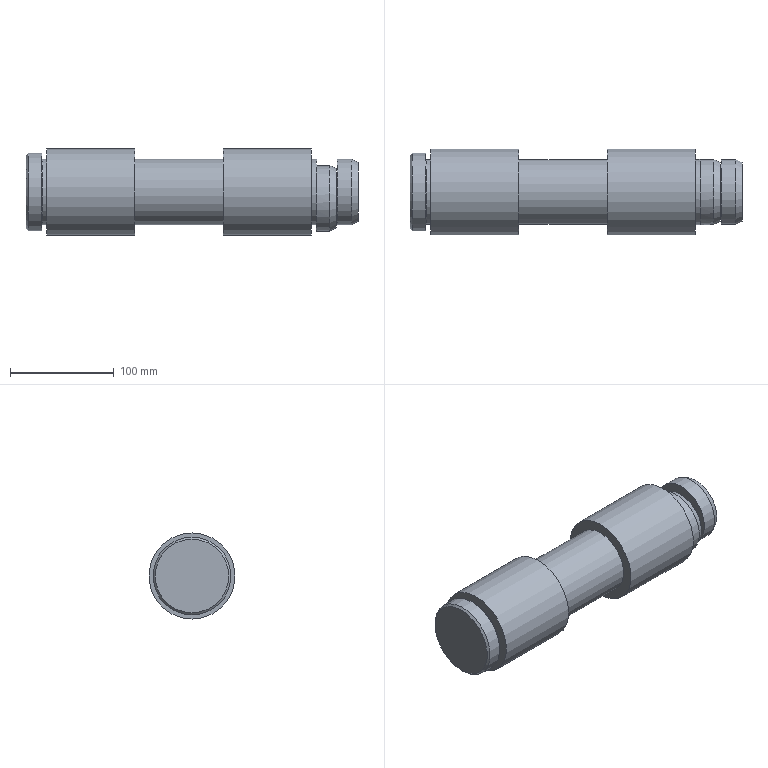Part | NX | features solid 2 | 1 solid | 36 faces | box 320 x 83 x 83 mm | volume 1384742 mm3 | plane 14 | cylinder 12 | cone 7 | torus 3 | commonest cylinder face diameters 63 x5 83 x2 27 x1 27.2 x1 32 x1 44 x1
STEP:
#1=CARTESIAN_POINT('',(-1305.,-953.648,-403.05));
#2=VERTEX_POINT('',#1);
#3=CARTESIAN_POINT('',(-1305.,-1016.352,-403.05));
#4=VERTEX_POINT('',#3);
#5=CARTESIAN_POINT('',(-1305.,-985.,-406.1));
#6=DIRECTION('',(1.,0.,0.));
#7=DIRECTION('',(0.,0.,-1.));
#8=AXIS2_PLACEMENT_3D('',#5,#6,#7);
#9=CIRCLE('',#8,31.5);
#10=EDGE_CURVE('',#2,#4,#9,.T.);
#11=ORIENTED_EDGE('',*,*,#10,.F.);
#12=CARTESIAN_POINT('',(-1305.,-985.,-400.));
#13=DIRECTION('',(1.,0.,0.));
#14=DIRECTION('',(0.,0.,1.));
#15=AXIS2_PLACEMENT_3D('',#12,#13,#14);
#16=CIRCLE('',#15,31.5);
#17=EDGE_CURVE('',#2,#4,#16,.T.);
#18=ORIENTED_EDGE('',*,*,#17,.T.);
#19=EDGE_LOOP('',(#11,#18));
#20=FACE_BOUND('',#19,.T.);
#21=CARTESIAN_POINT('',(-1305.,-985.,-400.));
#22=DIRECTION('',(1.,0.,0.));
#23=DIRECTION('',(0.,0.,1.));
#24=AXIS2_PLACEMENT_3D('',#21,#22,#23);
#25=PLANE('',#24);
#26=ADVANCED_FACE('',(#20),#25,.T.);
#27=CARTESIAN_POINT('',(-1310.,-985.,-431.5));
#28=VERTEX_POINT('',#27);
#29=CARTESIAN_POINT('',(-1310.,-985.,-400.));
#30=DIRECTION('',(1.,0.,0.));
#31=DIRECTION('',(0.,0.,-1.));
#32=AXIS2_PLACEMENT_3D('',#29,#30,#31);
#33=CIRCLE('',#32,31.5);
#34=EDGE_CURVE('',#28,#28,#33,.F.);
#35=ORIENTED_EDGE('',*,*,#34,.F.);
#36=EDGE_LOOP('',(#35));
#37=FACE_BOUND('',#36,.T.);
#38=CARTESIAN_POINT('',(-1305.,-985.,-400.));
#39=DIRECTION('',(1.,0.,0.));
#40=DIRECTION('',(0.,0.,1.));
#41=AXIS2_PLACEMENT_3D('',#38,#39,#40);
#42=CIRCLE('',#41,31.5);
#43=EDGE_CURVE('',#4,#2,#42,.T.);
#44=ORIENTED_EDGE('',*,*,#43,.F.);
#45=ORIENTED_EDGE('',*,*,#17,.F.);
#46=EDGE_LOOP('',(#44,#45));
#47=FACE_BOUND('',#46,.T.);
#48=CARTESIAN_POINT('',(-1570.,-985.,-400.));
#49=DIRECTION('',(1.,0.,0.));
#50=DIRECTION('',(0.,0.,1.));
#51=AXIS2_PLACEMENT_3D('',#48,#49,#50);
#52=CYLINDRICAL_SURFACE('',#51,31.5);
#53=ADVANCED_FACE('',(#37,#47),#52,.T.);
#54=ORIENTED_EDGE('',*,*,#34,.T.);
#55=EDGE_LOOP('',(#54));
#56=FACE_BOUND('',#55,.T.);
#57=CARTESIAN_POINT('',(-1310.,-985.,-441.5));
#58=VERTEX_POINT('',#57);
#59=CARTESIAN_POINT('',(-1310.,-985.,-400.));
#60=DIRECTION('',(-1.,0.,0.));
#61=DIRECTION('',(0.,0.,-1.));
#62=AXIS2_PLACEMENT_3D('',#59,#60,#61);
#63=CIRCLE('',#62,41.5);
#64=EDGE_CURVE('',#58,#58,#63,.T.);
#65=ORIENTED_EDGE('',*,*,#64,.F.);
#66=EDGE_LOOP('',(#65));
#67=FACE_BOUND('',#66,.T.);
#68=CARTESIAN_POINT('',(-1310.,-985.,-400.));
#69=DIRECTION('',(1.,0.,0.));
#70=DIRECTION('',(0.,0.,1.));
#71=AXIS2_PLACEMENT_3D('',#68,#69,#70);
#72=PLANE('',#71);
#73=ADVANCED_FACE('',(#56,#67),#72,.T.);
#74=CARTESIAN_POINT('',(-1395.,-985.,-368.5));
#75=VERTEX_POINT('',#74);
#76=CARTESIAN_POINT('',(-1395.,-985.,-400.));
#77=DIRECTION('',(-1.,0.,0.));
#78=DIRECTION('',(0.,0.,1.));
#79=AXIS2_PLACEMENT_3D('',#76,#77,#78);
#80=CIRCLE('',#79,31.5);
#81=EDGE_CURVE('',#75,#75,#80,.F.);
#82=ORIENTED_EDGE('',*,*,#81,.T.);
#83=EDGE_LOOP('',(#82));
#84=FACE_BOUND('',#83,.T.);
#85=CARTESIAN_POINT('',(-1395.,-985.,-358.5));
#86=VERTEX_POINT('',#85);
#87=CARTESIAN_POINT('',(-1395.,-985.,-400.));
#88=DIRECTION('',(1.,0.,0.));
#89=DIRECTION('',(0.,0.,1.));
#90=AXIS2_PLACEMENT_3D('',#87,#88,#89);
#91=CIRCLE('',#90,41.5);
#92=EDGE_CURVE('',#86,#86,#91,.T.);
#93=ORIENTED_EDGE('',*,*,#92,.F.);
#94=EDGE_LOOP('',(#93));
#95=FACE_BOUND('',#94,.T.);
#96=CARTESIAN_POINT('',(-1395.,-985.,-400.));
#97=DIRECTION('',(-1.,0.,0.));
#98=DIRECTION('',(0.,0.,-1.));
#99=AXIS2_PLACEMENT_3D('',#96,#97,#98);
#100=PLANE('',#99);
#101=ADVANCED_FACE('',(#84,#95),#100,.T.);
#102=ORIENTED_EDGE('',*,*,#64,.T.);
#103=EDGE_LOOP('',(#102));
#104=FACE_BOUND('',#103,.T.);
#105=ORIENTED_EDGE('',*,*,#92,.T.);
#106=EDGE_LOOP('',(#105));
#107=FACE_BOUND('',#106,.T.);
#108=CARTESIAN_POINT('',(-1395.,-985.,-400.));
#109=DIRECTION('',(1.,0.,0.));
#110=DIRECTION('',(0.,0.,1.));
#111=AXIS2_PLACEMENT_3D('',#108,#109,#110);
#112=CYLINDRICAL_SURFACE('',#111,41.5);
#113=ADVANCED_FACE('',(#104,#107),#112,.T.);
#114=CARTESIAN_POINT('',(-1585.,-985.,-364.5));
#115=VERTEX_POINT('',#114);
#116=CARTESIAN_POINT('',(-1585.,-985.,-400.));
#117=DIRECTION('',(-1.,0.,0.));
#118=DIRECTION('',(0.,0.,1.));
#119=AXIS2_PLACEMENT_3D('',#116,#117,#118);
#120=CIRCLE('',#119,35.5);
#121=EDGE_CURVE('',#115,#115,#120,.T.);
#122=ORIENTED_EDGE('',*,*,#121,.T.);
#123=EDGE_LOOP('',(#122));
#124=FACE_BOUND('',#123,.T.);
#125=CARTESIAN_POINT('',(-1585.,-985.,-400.));
#126=DIRECTION('',(-1.,0.,0.));
#127=DIRECTION('',(0.,0.,-1.));
#128=AXIS2_PLACEMENT_3D('',#125,#126,#127);
#129=PLANE('',#128);
#130=ADVANCED_FACE('',(#124),#129,.T.);
#131=ORIENTED_EDGE('',*,*,#121,.F.);
#132=EDGE_LOOP('',(#131));
#133=FACE_BOUND('',#132,.T.);
#134=CARTESIAN_POINT('',(-1583.,-985.,-362.5));
#135=VERTEX_POINT('',#134);
#136=CARTESIAN_POINT('',(-1583.,-985.,-400.));
#137=DIRECTION('',(-1.,0.,0.));
#138=DIRECTION('',(0.,0.,1.));
#139=AXIS2_PLACEMENT_3D('',#136,#137,#138);
#140=CIRCLE('',#139,37.5);
#141=EDGE_CURVE('',#135,#135,#140,.F.);
#142=ORIENTED_EDGE('',*,*,#141,.F.);
#143=EDGE_LOOP('',(#142));
#144=FACE_BOUND('',#143,.T.);
#145=CARTESIAN_POINT('',(-1583.,-985.,-400.));
#146=DIRECTION('',(1.,0.,0.));
#147=DIRECTION('',(0.,0.,-1.));
#148=AXIS2_PLACEMENT_3D('',#145,#146,#147);
#149=CONICAL_SURFACE('',#148,37.5,0.7854);
#150=ADVANCED_FACE('',(#133,#144),#149,.T.);
#151=ORIENTED_EDGE('',*,*,#141,.T.);
#152=EDGE_LOOP('',(#151));
#153=FACE_BOUND('',#152,.T.);
#154=CARTESIAN_POINT('',(-1570.,-985.,-437.5));
#155=VERTEX_POINT('',#154);
#156=CARTESIAN_POINT('',(-1570.,-985.,-400.));
#157=DIRECTION('',(-1.,0.,0.));
#158=DIRECTION('',(0.,0.,-1.));
#159=AXIS2_PLACEMENT_3D('',#156,#157,#158);
#160=CIRCLE('',#159,37.5);
#161=EDGE_CURVE('',#155,#155,#160,.T.);
#162=ORIENTED_EDGE('',*,*,#161,.T.);
#163=EDGE_LOOP('',(#162));
#164=FACE_BOUND('',#163,.T.);
#165=CARTESIAN_POINT('',(-1585.,-985.,-400.));
#166=DIRECTION('',(1.,0.,0.));
#167=DIRECTION('',(0.,0.,1.));
#168=AXIS2_PLACEMENT_3D('',#165,#166,#167);
#169=CYLINDRICAL_SURFACE('',#168,37.5);
#170=ADVANCED_FACE('',(#153,#164),#169,.T.);
#171=CARTESIAN_POINT('',(-1570.,-985.,-432.5));
#172=VERTEX_POINT('',#171);
#173=CARTESIAN_POINT('',(-1570.,-985.,-400.));
#174=DIRECTION('',(1.,0.,0.));
#175=DIRECTION('',(0.,0.,-1.));
#176=AXIS2_PLACEMENT_3D('',#173,#174,#175);
#177=CIRCLE('',#176,32.5);
#178=EDGE_CURVE('',#172,#172,#177,.F.);
#179=ORIENTED_EDGE('',*,*,#178,.T.);
#180=EDGE_LOOP('',(#179));
#181=FACE_BOUND('',#180,.T.);
#182=ORIENTED_EDGE('',*,*,#161,.F.);
#183=EDGE_LOOP('',(#182));
#184=FACE_BOUND('',#183,.T.);
#185=CARTESIAN_POINT('',(-1570.,-985.,-400.));
#186=DIRECTION('',(1.,0.,0.));
#187=DIRECTION('',(0.,0.,1.));
#188=AXIS2_PLACEMENT_3D('',#185,#186,#187);
#189=PLANE('',#188);
#190=ADVANCED_FACE('',(#181,#184),#189,.T.);
#191=ORIENTED_EDGE('',*,*,#178,.F.);
#192=EDGE_LOOP('',(#191));
#193=FACE_BOUND('',#192,.T.);
#194=CARTESIAN_POINT('',(-1569.,-985.,-431.5));
#195=VERTEX_POINT('',#194);
#196=CARTESIAN_POINT('',(-1569.,-985.,-400.));
#197=DIRECTION('',(1.,0.,0.));
#198=DIRECTION('',(0.,0.,-1.));
#199=AXIS2_PLACEMENT_3D('',#196,#197,#198);
#200=CIRCLE('',#199,31.5);
#201=EDGE_CURVE('',#195,#195,#200,.T.);
#202=ORIENTED_EDGE('',*,*,#201,.F.);
#203=EDGE_LOOP('',(#202));
#204=FACE_BOUND('',#203,.T.);
#205=CARTESIAN_POINT('',(-1569.,-985.,-400.));
#206=DIRECTION('',(1.,0.,0.));
#207=DIRECTION('',(0.,0.,-1.));
#208=AXIS2_PLACEMENT_3D('',#205,#206,#207);
#209=TOROIDAL_SURFACE('',#208,32.5,1.);
#210=ADVANCED_FACE('',(#193,#204),#209,.F.);
#211=CARTESIAN_POINT('',(-1565.,-985.,-368.5));
#212=VERTEX_POINT('',#211);
#213=CARTESIAN_POINT('',(-1565.,-985.,-400.));
#214=DIRECTION('',(-1.,0.,0.));
#215=DIRECTION('',(0.,0.,1.));
#216=AXIS2_PLACEMENT_3D('',#213,#214,#215);
#217=CIRCLE('',#216,31.5);
#218=EDGE_CURVE('',#212,#212,#217,.F.);
#219=ORIENTED_EDGE('',*,*,#218,.F.);
#220=EDGE_LOOP('',(#219));
#221=FACE_BOUND('',#220,.T.);
#222=ORIENTED_EDGE('',*,*,#201,.T.);
#223=EDGE_LOOP('',(#222));
#224=FACE_BOUND('',#223,.T.);
#225=CARTESIAN_POINT('',(-1570.,-985.,-400.));
#226=DIRECTION('',(1.,0.,0.));
#227=DIRECTION('',(0.,0.,1.));
#228=AXIS2_PLACEMENT_3D('',#225,#226,#227);
#229=CYLINDRICAL_SURFACE('',#228,31.5);
#230=ADVANCED_FACE('',(#221,#224),#229,.T.);
#231=ORIENTED_EDGE('',*,*,#218,.T.);
#232=EDGE_LOOP('',(#231));
#233=FACE_BOUND('',#232,.T.);
#234=CARTESIAN_POINT('',(-1565.,-985.,-358.5));
#235=VERTEX_POINT('',#234);
#236=CARTESIAN_POINT('',(-1565.,-985.,-400.));
#237=DIRECTION('',(1.,0.,0.));
#238=DIRECTION('',(0.,0.,1.));
#239=AXIS2_PLACEMENT_3D('',#236,#237,#238);
#240=CIRCLE('',#239,41.5);
#241=EDGE_CURVE('',#235,#235,#240,.T.);
#242=ORIENTED_EDGE('',*,*,#241,.F.);
#243=EDGE_LOOP('',(#242));
#244=FACE_BOUND('',#243,.T.);
#245=CARTESIAN_POINT('',(-1565.,-985.,-400.));
#246=DIRECTION('',(-1.,0.,0.));
#247=DIRECTION('',(0.,0.,-1.));
#248=AXIS2_PLACEMENT_3D('',#245,#246,#247);
#249=PLANE('',#248);
#250=ADVANCED_FACE('',(#233,#244),#249,.T.);
#251=CARTESIAN_POINT('',(-1480.,-985.,-441.5));
#252=VERTEX_POINT('',#251);
#253=CARTESIAN_POINT('',(-1480.,-985.,-400.));
#254=DIRECTION('',(-1.,0.,0.));
#255=DIRECTION('',(0.,0.,-1.));
#256=AXIS2_PLACEMENT_3D('',#253,#254,#255);
#257=CIRCLE('',#256,41.5);
#258=EDGE_CURVE('',#252,#252,#257,.T.);
#259=ORIENTED_EDGE('',*,*,#258,.T.);
#260=EDGE_LOOP('',(#259));
#261=FACE_BOUND('',#260,.T.);
#262=ORIENTED_EDGE('',*,*,#241,.T.);
#263=EDGE_LOOP('',(#262));
#264=FACE_BOUND('',#263,.T.);
#265=CARTESIAN_POINT('',(-1565.,-985.,-400.));
#266=DIRECTION('',(1.,0.,0.));
#267=DIRECTION('',(0.,0.,1.));
#268=AXIS2_PLACEMENT_3D('',#265,#266,#267);
#269=CYLINDRICAL_SURFACE('',#268,41.5);
#270=ADVANCED_FACE('',(#261,#264),#269,.T.);
#271=CARTESIAN_POINT('',(-1480.,-985.,-431.5));
#272=VERTEX_POINT('',#271);
#273=CARTESIAN_POINT('',(-1480.,-985.,-400.));
#274=DIRECTION('',(1.,0.,0.));
#275=DIRECTION('',(0.,0.,-1.));
#276=AXIS2_PLACEMENT_3D('',#273,#274,#275);
#277=CIRCLE('',#276,31.5);
#278=EDGE_CURVE('',#272,#272,#277,.F.);
#279=ORIENTED_EDGE('',*,*,#278,.T.);
#280=EDGE_LOOP('',(#279));
#281=FACE_BOUND('',#280,.T.);
#282=ORIENTED_EDGE('',*,*,#258,.F.);
#283=EDGE_LOOP('',(#282));
#284=FACE_BOUND('',#283,.T.);
#285=CARTESIAN_POINT('',(-1480.,-985.,-400.));
#286=DIRECTION('',(1.,0.,0.));
#287=DIRECTION('',(0.,0.,1.));
#288=AXIS2_PLACEMENT_3D('',#285,#286,#287);
#289=PLANE('',#288);
#290=ADVANCED_FACE('',(#281,#284),#289,.T.);
#291=ORIENTED_EDGE('',*,*,#81,.F.);
#292=EDGE_LOOP('',(#291));
#293=FACE_BOUND('',#292,.T.);
#294=ORIENTED_EDGE('',*,*,#278,.F.);
#295=EDGE_LOOP('',(#294));
#296=FACE_BOUND('',#295,.T.);
#297=CARTESIAN_POINT('',(-1570.,-985.,-400.));
#298=DIRECTION('',(1.,0.,0.));
#299=DIRECTION('',(0.,0.,1.));
#300=AXIS2_PLACEMENT_3D('',#297,#298,#299);
#301=CYLINDRICAL_SURFACE('',#300,31.5);
#302=ADVANCED_FACE('',(#293,#296),#301,.T.);
#303=CARTESIAN_POINT('',(-1286.,-985.,-434.6));
#304=VERTEX_POINT('',#303);
#305=CARTESIAN_POINT('',(-1286.,-985.,-406.1));
#306=DIRECTION('',(1.,0.,0.));
#307=DIRECTION('',(0.,0.,-1.));
#308=AXIS2_PLACEMENT_3D('',#305,#306,#307);
#309=CIRCLE('',#308,28.5);
#310=EDGE_CURVE('',#304,#304,#309,.T.);
#311=ORIENTED_EDGE('',*,*,#310,.T.);
#312=EDGE_LOOP('',(#311));
#313=FACE_BOUND('',#312,.T.);
#314=CARTESIAN_POINT('',(-1286.,-981.618,-384.361));
#315=VERTEX_POINT('',#314);
#316=CARTESIAN_POINT('',(-1286.,-988.382,-384.361));
#317=VERTEX_POINT('',#316);
#318=CARTESIAN_POINT('',(-1286.,-985.,-406.1));
#319=DIRECTION('',(-1.,0.,0.));
#320=DIRECTION('',(0.,0.,-1.));
#321=AXIS2_PLACEMENT_3D('',#318,#319,#320);
#322=CIRCLE('',#321,22.);
#323=EDGE_CURVE('',#315,#317,#322,.T.);
#324=ORIENTED_EDGE('',*,*,#323,.T.);
#325=CARTESIAN_POINT('',(-1286.,-985.,-400.));
#326=DIRECTION('',(1.,0.,0.));
#327=DIRECTION('',(0.,0.,-1.));
#328=AXIS2_PLACEMENT_3D('',#325,#326,#327);
#329=CIRCLE('',#328,16.);
#330=EDGE_CURVE('',#317,#315,#329,.F.);
#331=ORIENTED_EDGE('',*,*,#330,.T.);
#332=EDGE_LOOP('',(#324,#331));
#333=FACE_BOUND('',#332,.T.);
#334=CARTESIAN_POINT('',(-1286.,-985.,-406.1));
#335=DIRECTION('',(1.,0.,0.));
#336=DIRECTION('',(0.,0.,1.));
#337=AXIS2_PLACEMENT_3D('',#334,#335,#336);
#338=PLANE('',#337);
#339=ADVANCED_FACE('',(#313,#333),#338,.T.);
#340=CARTESIAN_POINT('',(-1305.,-985.,-406.1));
#341=DIRECTION('',(1.,0.,0.));
#342=DIRECTION('',(0.,0.,1.));
#343=AXIS2_PLACEMENT_3D('',#340,#341,#342);
#344=CIRCLE('',#343,31.5);
#345=EDGE_CURVE('',#4,#2,#344,.T.);
#346=ORIENTED_EDGE('',*,*,#345,.F.);
#347=ORIENTED_EDGE('',*,*,#43,.T.);
#348=EDGE_LOOP('',(#346,#347));
#349=FACE_BOUND('',#348,.T.);
#350=CARTESIAN_POINT('',(-1305.,-985.,-406.1));
#351=DIRECTION('',(-1.,0.,0.));
#352=DIRECTION('',(0.,0.,-1.));
#353=AXIS2_PLACEMENT_3D('',#350,#351,#352);
#354=PLANE('',#353);
#355=ADVANCED_FACE('',(#349),#354,.T.);
#356=CARTESIAN_POINT('',(-1292.,-985.,-437.6));
#357=VERTEX_POINT('',#356);
#358=CARTESIAN_POINT('',(-1292.,-985.,-406.1));
#359=DIRECTION('',(1.,0.,0.));
#360=DIRECTION('',(0.,0.,-1.));
#361=AXIS2_PLACEMENT_3D('',#358,#359,#360);
#362=CIRCLE('',#361,31.5);
#363=EDGE_CURVE('',#357,#357,#362,.F.);
#364=ORIENTED_EDGE('',*,*,#363,.T.);
#365=EDGE_LOOP('',(#364));
#366=FACE_BOUND('',#365,.T.);
#367=ORIENTED_EDGE('',*,*,#345,.T.);
#368=ORIENTED_EDGE('',*,*,#10,.T.);
#369=EDGE_LOOP('',(#367,#368));
#370=FACE_BOUND('',#369,.T.);
#371=CARTESIAN_POINT('',(-1305.,-985.,-406.1));
#372=DIRECTION('',(1.,0.,0.));
#373=DIRECTION('',(0.,0.,1.));
#374=AXIS2_PLACEMENT_3D('',#371,#372,#373);
#375=CYLINDRICAL_SURFACE('',#374,31.5);
#376=ADVANCED_FACE('',(#366,#370),#375,.T.);
#377=CARTESIAN_POINT('',(-1304.2,-981.618,-384.361));
#378=VERTEX_POINT('',#377);
#379=CARTESIAN_POINT('',(-1295.1,-981.618,-384.361));
#380=DIRECTION('',(-1.,0.,0.));
#381=VECTOR('',#380,1000.);
#382=LINE('',#379,#381);
#383=EDGE_CURVE('',#378,#315,#382,.F.);
#384=ORIENTED_EDGE('',*,*,#383,.F.);
#385=CARTESIAN_POINT('',(-1304.2,-988.382,-384.361));
#386=VERTEX_POINT('',#385);
#387=CARTESIAN_POINT('',(-1304.2,-985.,-406.1));
#388=DIRECTION('',(-1.,0.,0.));
#389=DIRECTION('',(0.,0.,1.));
#390=AXIS2_PLACEMENT_3D('',#387,#388,#389);
#391=CIRCLE('',#390,22.);
#392=EDGE_CURVE('',#378,#386,#391,.T.);
#393=ORIENTED_EDGE('',*,*,#392,.T.);
#394=CARTESIAN_POINT('',(-1295.1,-988.382,-384.361));
#395=DIRECTION('',(-1.,0.,0.));
#396=VECTOR('',#395,1000.);
#397=LINE('',#394,#396);
#398=EDGE_CURVE('',#317,#386,#397,.T.);
#399=ORIENTED_EDGE('',*,*,#398,.F.);
#400=ORIENTED_EDGE('',*,*,#323,.F.);
#401=EDGE_LOOP('',(#384,#393,#399,#400));
#402=FACE_BOUND('',#401,.T.);
#403=CARTESIAN_POINT('',(-1286.,-985.,-406.1));
#404=DIRECTION('',(-1.,0.,0.));
#405=DIRECTION('',(0.,0.,-1.));
#406=AXIS2_PLACEMENT_3D('',#403,#404,#405);
#407=CYLINDRICAL_SURFACE('',#406,22.);
#408=ADVANCED_FACE('',(#402),#407,.F.);
#409=CARTESIAN_POINT('',(-1305.,-985.,-428.9));
#410=VERTEX_POINT('',#409);
#411=CARTESIAN_POINT('',(-1305.,-985.,-406.1));
#412=DIRECTION('',(1.,0.,0.));
#413=DIRECTION('',(0.,0.,-1.));
#414=AXIS2_PLACEMENT_3D('',#411,#412,#413);
#415=CIRCLE('',#414,22.8);
#416=EDGE_CURVE('',#410,#410,#415,.F.);
#417=ORIENTED_EDGE('',*,*,#416,.T.);
#418=EDGE_LOOP('',(#417));
#419=FACE_BOUND('',#418,.T.);
#420=ORIENTED_EDGE('',*,*,#392,.F.);
#421=CARTESIAN_POINT('',(-1304.2,-981.618,-384.361));
#422=CARTESIAN_POINT('',(-1304.334,-983.853,-383.878));
#423=CARTESIAN_POINT('',(-1304.334,-986.147,-383.878));
#424=CARTESIAN_POINT('',(-1304.2,-988.382,-384.361));
#425=B_SPLINE_CURVE_WITH_KNOTS('',3,(#421,#422,#423,#424),.UNSPECIFIED.,.F.,.F.,(4,4),(0.000003368,0.006776),.UNSPECIFIED.);
#426=EDGE_CURVE('',#378,#386,#425,.T.);
#427=ORIENTED_EDGE('',*,*,#426,.T.);
#428=EDGE_LOOP('',(#420,#427));
#429=FACE_BOUND('',#428,.T.);
#430=CARTESIAN_POINT('',(-1304.2,-985.,-406.1));
#431=DIRECTION('',(-1.,0.,0.));
#432=DIRECTION('',(0.,0.,1.));
#433=AXIS2_PLACEMENT_3D('',#430,#431,#432);
#434=CONICAL_SURFACE('',#433,22.,0.7854);
#435=ADVANCED_FACE('',(#419,#429),#434,.F.);
#436=ORIENTED_EDGE('',*,*,#310,.F.);
#437=EDGE_LOOP('',(#436));
#438=FACE_BOUND('',#437,.T.);
#439=ORIENTED_EDGE('',*,*,#363,.F.);
#440=EDGE_LOOP('',(#439));
#441=FACE_BOUND('',#440,.T.);
#442=CARTESIAN_POINT('',(-1292.,-985.,-406.1));
#443=DIRECTION('',(-1.,0.,0.));
#444=DIRECTION('',(0.,0.,1.));
#445=AXIS2_PLACEMENT_3D('',#442,#443,#444);
#446=CONICAL_SURFACE('',#445,31.5,0.4636);
#447=ADVANCED_FACE('',(#438,#441),#446,.T.);
#448=CARTESIAN_POINT('',(-1265.,-985.,-408.5));
#449=VERTEX_POINT('',#448);
#450=CARTESIAN_POINT('',(-1265.,-985.,-400.));
#451=DIRECTION('',(1.,0.,0.));
#452=DIRECTION('',(0.,0.,-1.));
#453=AXIS2_PLACEMENT_3D('',#450,#451,#452);
#454=CIRCLE('',#453,8.5);
#455=EDGE_CURVE('',#449,#449,#454,.T.);
#456=ORIENTED_EDGE('',*,*,#455,.T.);
#457=EDGE_LOOP('',(#456));
#458=FACE_BOUND('',#457,.T.);
#459=CARTESIAN_POINT('',(-1265.,-985.,-400.));
#460=DIRECTION('',(1.,0.,0.));
#461=DIRECTION('',(0.,0.,1.));
#462=AXIS2_PLACEMENT_3D('',#459,#460,#461);
#463=PLANE('',#462);
#464=ADVANCED_FACE('',(#458),#463,.T.);
#465=CARTESIAN_POINT('',(-1270.,-985.,-413.5));
#466=VERTEX_POINT('',#465);
#467=CARTESIAN_POINT('',(-1270.,-985.,-400.));
#468=DIRECTION('',(1.,0.,0.));
#469=DIRECTION('',(0.,0.,-1.));
#470=AXIS2_PLACEMENT_3D('',#467,#468,#469);
#471=CIRCLE('',#470,13.5);
#472=EDGE_CURVE('',#466,#466,#471,.F.);
#473=ORIENTED_EDGE('',*,*,#472,.F.);
#474=EDGE_LOOP('',(#473));
#475=FACE_BOUND('',#474,.T.);
#476=ORIENTED_EDGE('',*,*,#455,.F.);
#477=EDGE_LOOP('',(#476));
#478=FACE_BOUND('',#477,.T.);
#479=CARTESIAN_POINT('',(-1265.,-985.,-400.));
#480=DIRECTION('',(-1.,0.,0.));
#481=DIRECTION('',(0.,0.,1.));
#482=AXIS2_PLACEMENT_3D('',#479,#480,#481);
#483=CONICAL_SURFACE('',#482,8.5,0.7854);
#484=ADVANCED_FACE('',(#475,#478),#483,.T.);
#485=CARTESIAN_POINT('',(-1284.4,-985.,-413.5));
#486=VERTEX_POINT('',#485);
#487=CARTESIAN_POINT('',(-1284.4,-985.,-400.));
#488=DIRECTION('',(1.,0.,0.));
#489=DIRECTION('',(0.,0.,-1.));
#490=AXIS2_PLACEMENT_3D('',#487,#488,#489);
#491=CIRCLE('',#490,13.5);
#492=EDGE_CURVE('',#486,#486,#491,.T.);
#493=ORIENTED_EDGE('',*,*,#492,.T.);
#494=EDGE_LOOP('',(#493));
#495=FACE_BOUND('',#494,.T.);
#496=ORIENTED_EDGE('',*,*,#472,.T.);
#497=EDGE_LOOP('',(#496));
#498=FACE_BOUND('',#497,.T.);
#499=CARTESIAN_POINT('',(-1285.,-985.,-400.));
#500=DIRECTION('',(1.,0.,0.));
#501=DIRECTION('',(0.,0.,1.));
#502=AXIS2_PLACEMENT_3D('',#499,#500,#501);
#503=CYLINDRICAL_SURFACE('',#502,13.5);
#504=ADVANCED_FACE('',(#495,#498),#503,.T.);
#505=CARTESIAN_POINT('',(-1285.,-985.,-414.1));
#506=VERTEX_POINT('',#505);
#507=CARTESIAN_POINT('',(-1285.,-985.,-400.));
#508=DIRECTION('',(1.,0.,0.));
#509=DIRECTION('',(0.,0.,-1.));
#510=AXIS2_PLACEMENT_3D('',#507,#508,#509);
#511=CIRCLE('',#510,14.1);
#512=EDGE_CURVE('',#506,#506,#511,.F.);
#513=ORIENTED_EDGE('',*,*,#512,.F.);
#514=EDGE_LOOP('',(#513));
#515=FACE_BOUND('',#514,.T.);
#516=ORIENTED_EDGE('',*,*,#492,.F.);
#517=EDGE_LOOP('',(#516));
#518=FACE_BOUND('',#517,.T.);
#519=CARTESIAN_POINT('',(-1284.4,-985.,-400.));
#520=DIRECTION('',(1.,0.,0.));
#521=DIRECTION('',(0.,0.,-1.));
#522=AXIS2_PLACEMENT_3D('',#519,#520,#521);
#523=TOROIDAL_SURFACE('',#522,14.1,0.6);
#524=ADVANCED_FACE('',(#515,#518),#523,.F.);
#525=CARTESIAN_POINT('',(-1285.,-985.,-414.4));
#526=VERTEX_POINT('',#525);
#527=CARTESIAN_POINT('',(-1285.,-985.,-400.));
#528=DIRECTION('',(1.,0.,0.));
#529=DIRECTION('',(0.,0.,-1.));
#530=AXIS2_PLACEMENT_3D('',#527,#528,#529);
#531=CIRCLE('',#530,14.4);
#532=EDGE_CURVE('',#526,#526,#531,.F.);
#533=ORIENTED_EDGE('',*,*,#532,.F.);
#534=EDGE_LOOP('',(#533));
#535=FACE_BOUND('',#534,.T.);
#536=ORIENTED_EDGE('',*,*,#512,.T.);
#537=EDGE_LOOP('',(#536));
#538=FACE_BOUND('',#537,.T.);
#539=CARTESIAN_POINT('',(-1285.,-985.,-400.));
#540=DIRECTION('',(1.,0.,0.));
#541=DIRECTION('',(0.,0.,1.));
#542=AXIS2_PLACEMENT_3D('',#539,#540,#541);
#543=PLANE('',#542);
#544=ADVANCED_FACE('',(#535,#538),#543,.T.);
#545=ORIENTED_EDGE('',*,*,#532,.T.);
#546=EDGE_LOOP('',(#545));
#547=FACE_BOUND('',#546,.T.);
#548=CARTESIAN_POINT('',(-1284.2,-985.,-386.4));
#549=VERTEX_POINT('',#548);
#550=CARTESIAN_POINT('',(-1284.2,-985.,-400.));
#551=DIRECTION('',(-1.,0.,0.));
#552=DIRECTION('',(0.,0.,1.));
#553=AXIS2_PLACEMENT_3D('',#550,#551,#552);
#554=CIRCLE('',#553,13.6);
#555=EDGE_CURVE('',#549,#549,#554,.T.);
#556=ORIENTED_EDGE('',*,*,#555,.F.);
#557=EDGE_LOOP('',(#556));
#558=FACE_BOUND('',#557,.T.);
#559=CARTESIAN_POINT('',(-1284.2,-985.,-400.));
#560=DIRECTION('',(-1.,0.,0.));
#561=DIRECTION('',(0.,0.,1.));
#562=AXIS2_PLACEMENT_3D('',#559,#560,#561);
#563=CONICAL_SURFACE('',#562,13.6,0.7854);
#564=ADVANCED_FACE('',(#547,#558),#563,.F.);
#565=ORIENTED_EDGE('',*,*,#555,.T.);
#566=EDGE_LOOP('',(#565));
#567=FACE_BOUND('',#566,.T.);
#568=CARTESIAN_POINT('',(-1270.,-985.,-413.6));
#569=VERTEX_POINT('',#568);
#570=CARTESIAN_POINT('',(-1270.,-985.,-400.));
#571=DIRECTION('',(1.,0.,0.));
#572=DIRECTION('',(0.,0.,-1.));
#573=AXIS2_PLACEMENT_3D('',#570,#571,#572);
#574=CIRCLE('',#573,13.6);
#575=EDGE_CURVE('',#569,#569,#574,.T.);
#576=ORIENTED_EDGE('',*,*,#575,.T.);
#577=EDGE_LOOP('',(#576));
#578=FACE_BOUND('',#577,.T.);
#579=CARTESIAN_POINT('',(-1265.,-985.,-400.));
#580=DIRECTION('',(-1.,0.,0.));
#581=DIRECTION('',(0.,0.,-1.));
#582=AXIS2_PLACEMENT_3D('',#579,#580,#581);
#583=CYLINDRICAL_SURFACE('',#582,13.6);
#584=ADVANCED_FACE('',(#567,#578),#583,.F.);
#585=ORIENTED_EDGE('',*,*,#575,.F.);
#586=EDGE_LOOP('',(#585));
#587=FACE_BOUND('',#586,.T.);
#588=CARTESIAN_POINT('',(-1265.,-985.,-418.6));
#589=VERTEX_POINT('',#588);
#590=CARTESIAN_POINT('',(-1265.,-985.,-400.));
#591=DIRECTION('',(1.,0.,0.));
#592=DIRECTION('',(0.,0.,-1.));
#593=AXIS2_PLACEMENT_3D('',#590,#591,#592);
#594=CIRCLE('',#593,18.6);
#595=EDGE_CURVE('',#589,#589,#594,.F.);
#596=ORIENTED_EDGE('',*,*,#595,.F.);
#597=EDGE_LOOP('',(#596));
#598=FACE_BOUND('',#597,.T.);
#599=CARTESIAN_POINT('',(-1265.,-985.,-400.));
#600=DIRECTION('',(1.,0.,0.));
#601=DIRECTION('',(0.,0.,-1.));
#602=AXIS2_PLACEMENT_3D('',#599,#600,#601);
#603=CONICAL_SURFACE('',#602,18.6,0.7854);
#604=ADVANCED_FACE('',(#587,#598),#603,.F.);
#605=CARTESIAN_POINT('',(-1265.,-985.,-428.5));
#606=VERTEX_POINT('',#605);
#607=CARTESIAN_POINT('',(-1265.,-985.,-400.));
#608=DIRECTION('',(1.,0.,0.));
#609=DIRECTION('',(0.,0.,-1.));
#610=AXIS2_PLACEMENT_3D('',#607,#608,#609);
#611=CIRCLE('',#610,28.5);
#612=EDGE_CURVE('',#606,#606,#611,.T.);
#613=ORIENTED_EDGE('',*,*,#612,.T.);
#614=EDGE_LOOP('',(#613));
#615=FACE_BOUND('',#614,.T.);
#616=ORIENTED_EDGE('',*,*,#595,.T.);
#617=EDGE_LOOP('',(#616));
#618=FACE_BOUND('',#617,.T.);
#619=CARTESIAN_POINT('',(-1265.,-985.,-400.));
#620=DIRECTION('',(1.,0.,0.));
#621=DIRECTION('',(0.,0.,1.));
#622=AXIS2_PLACEMENT_3D('',#619,#620,#621);
#623=PLANE('',#622);
#624=ADVANCED_FACE('',(#615,#618),#623,.T.);
#625=ORIENTED_EDGE('',*,*,#612,.F.);
#626=EDGE_LOOP('',(#625));
#627=FACE_BOUND('',#626,.T.);
#628=CARTESIAN_POINT('',(-1271.,-985.,-431.5));
#629=VERTEX_POINT('',#628);
#630=CARTESIAN_POINT('',(-1271.,-985.,-400.));
#631=DIRECTION('',(1.,0.,0.));
#632=DIRECTION('',(0.,0.,-1.));
#633=AXIS2_PLACEMENT_3D('',#630,#631,#632);
#634=CIRCLE('',#633,31.5);
#635=EDGE_CURVE('',#629,#629,#634,.F.);
#636=ORIENTED_EDGE('',*,*,#635,.F.);
#637=EDGE_LOOP('',(#636));
#638=FACE_BOUND('',#637,.T.);
#639=CARTESIAN_POINT('',(-1271.,-985.,-400.));
#640=DIRECTION('',(-1.,0.,0.));
#641=DIRECTION('',(0.,0.,1.));
#642=AXIS2_PLACEMENT_3D('',#639,#640,#641);
#643=CONICAL_SURFACE('',#642,31.5,0.4636);
#644=ADVANCED_FACE('',(#627,#638),#643,.T.);
#645=ORIENTED_EDGE('',*,*,#635,.T.);
#646=EDGE_LOOP('',(#645));
#647=FACE_BOUND('',#646,.T.);
#648=CARTESIAN_POINT('',(-1285.,-985.,-368.5));
#649=VERTEX_POINT('',#648);
#650=CARTESIAN_POINT('',(-1285.,-985.,-400.));
#651=DIRECTION('',(1.,0.,0.));
#652=DIRECTION('',(0.,0.,1.));
#653=AXIS2_PLACEMENT_3D('',#650,#651,#652);
#654=CIRCLE('',#653,31.5);
#655=EDGE_CURVE('',#649,#649,#654,.T.);
#656=ORIENTED_EDGE('',*,*,#655,.T.);
#657=EDGE_LOOP('',(#656));
#658=FACE_BOUND('',#657,.T.);
#659=CARTESIAN_POINT('',(-1285.,-985.,-400.));
#660=DIRECTION('',(1.,0.,0.));
#661=DIRECTION('',(0.,0.,1.));
#662=AXIS2_PLACEMENT_3D('',#659,#660,#661);
#663=CYLINDRICAL_SURFACE('',#662,31.5);
#664=ADVANCED_FACE('',(#647,#658),#663,.T.);
#665=CARTESIAN_POINT('',(-1285.,-985.,-384.));
#666=VERTEX_POINT('',#665);
#667=CARTESIAN_POINT('',(-1285.,-985.,-400.));
#668=DIRECTION('',(1.,0.,0.));
#669=DIRECTION('',(0.,0.,1.));
#670=AXIS2_PLACEMENT_3D('',#667,#668,#669);
#671=CIRCLE('',#670,16.);
#672=EDGE_CURVE('',#666,#666,#671,.T.);
#673=ORIENTED_EDGE('',*,*,#672,.T.);
#674=EDGE_LOOP('',(#673));
#675=FACE_BOUND('',#674,.T.);
#676=ORIENTED_EDGE('',*,*,#655,.F.);
#677=EDGE_LOOP('',(#676));
#678=FACE_BOUND('',#677,.T.);
#679=CARTESIAN_POINT('',(-1285.,-985.,-400.));
#680=DIRECTION('',(-1.,0.,0.));
#681=DIRECTION('',(0.,0.,-1.));
#682=AXIS2_PLACEMENT_3D('',#679,#680,#681);
#683=PLANE('',#682);
#684=ADVANCED_FACE('',(#675,#678),#683,.T.);
#685=ORIENTED_EDGE('',*,*,#416,.F.);
#686=EDGE_LOOP('',(#685));
#687=FACE_BOUND('',#686,.T.);
#688=CARTESIAN_POINT('',(-1305.,-985.,-416.6));
#689=VERTEX_POINT('',#688);
#690=CARTESIAN_POINT('',(-1305.,-985.,-400.));
#691=DIRECTION('',(1.,0.,0.));
#692=DIRECTION('',(0.,0.,-1.));
#693=AXIS2_PLACEMENT_3D('',#690,#691,#692);
#694=CIRCLE('',#693,16.6);
#695=EDGE_CURVE('',#689,#689,#694,.F.);
#696=ORIENTED_EDGE('',*,*,#695,.T.);
#697=EDGE_LOOP('',(#696));
#698=FACE_BOUND('',#697,.T.);
#699=CARTESIAN_POINT('',(-1305.,-985.,-400.));
#700=DIRECTION('',(1.,0.,0.));
#701=DIRECTION('',(0.,0.,1.));
#702=AXIS2_PLACEMENT_3D('',#699,#700,#701);
#703=PLANE('',#702);
#704=ADVANCED_FACE('',(#687,#698),#703,.T.);
#705=ORIENTED_EDGE('',*,*,#695,.F.);
#706=EDGE_LOOP('',(#705));
#707=FACE_BOUND('',#706,.T.);
#708=CARTESIAN_POINT('',(-1304.4,-985.,-416.));
#709=VERTEX_POINT('',#708);
#710=CARTESIAN_POINT('',(-1304.4,-985.,-400.));
#711=DIRECTION('',(1.,0.,0.));
#712=DIRECTION('',(0.,0.,-1.));
#713=AXIS2_PLACEMENT_3D('',#710,#711,#712);
#714=CIRCLE('',#713,16.);
#715=EDGE_CURVE('',#709,#709,#714,.T.);
#716=ORIENTED_EDGE('',*,*,#715,.F.);
#717=EDGE_LOOP('',(#716));
#718=FACE_BOUND('',#717,.T.);
#719=CARTESIAN_POINT('',(-1304.4,-985.,-400.));
#720=DIRECTION('',(1.,0.,0.));
#721=DIRECTION('',(0.,0.,-1.));
#722=AXIS2_PLACEMENT_3D('',#719,#720,#721);
#723=TOROIDAL_SURFACE('',#722,16.6,0.6);
#724=ADVANCED_FACE('',(#707,#718),#723,.F.);
#725=ORIENTED_EDGE('',*,*,#330,.F.);
#726=ORIENTED_EDGE('',*,*,#398,.T.);
#727=ORIENTED_EDGE('',*,*,#426,.F.);
#728=ORIENTED_EDGE('',*,*,#383,.T.);
#729=EDGE_LOOP('',(#725,#726,#727,#728));
#730=FACE_BOUND('',#729,.T.);
#731=ORIENTED_EDGE('',*,*,#715,.T.);
#732=EDGE_LOOP('',(#731));
#733=FACE_BOUND('',#732,.T.);
#734=ORIENTED_EDGE('',*,*,#672,.F.);
#735=EDGE_LOOP('',(#734));
#736=FACE_BOUND('',#735,.T.);
#737=CARTESIAN_POINT('',(-1305.,-985.,-400.));
#738=DIRECTION('',(1.,0.,0.));
#739=DIRECTION('',(0.,0.,1.));
#740=AXIS2_PLACEMENT_3D('',#737,#738,#739);
#741=CYLINDRICAL_SURFACE('',#740,16.);
#742=ADVANCED_FACE('',(#730,#733,#736),#741,.T.);
#743=CLOSED_SHELL('',(#26,#53,#73,#101,#113,#130,#150,#170,#190,#210,#230,#250,#270,#290,#302,#339,#355,#376,#408,#435,#447,#464,#484,#504,#524,#544,#564,#584,#604,#624,#644,#664,#684,#704,#724,#742));
#744=MANIFOLD_SOLID_BREP('',#743);
#745=(LENGTH_UNIT()NAMED_UNIT(*)SI_UNIT(.MILLI.,.METRE.));
#746=UNCERTAINTY_MEASURE_WITH_UNIT(LENGTH_MEASURE(0.0508),#745,'','');
#747=(NAMED_UNIT(*)PLANE_ANGLE_UNIT()SI_UNIT($,.RADIAN.));
#748=(NAMED_UNIT(*)SI_UNIT($,.STERADIAN.)SOLID_ANGLE_UNIT());
#749=(GEOMETRIC_REPRESENTATION_CONTEXT(3)GLOBAL_UNCERTAINTY_ASSIGNED_CONTEXT((#746))GLOBAL_UNIT_ASSIGNED_CONTEXT((#745,#747,#748))REPRESENTATION_CONTEXT('',''));
#750=ADVANCED_BREP_SHAPE_REPRESENTATION('',(#744),#749);